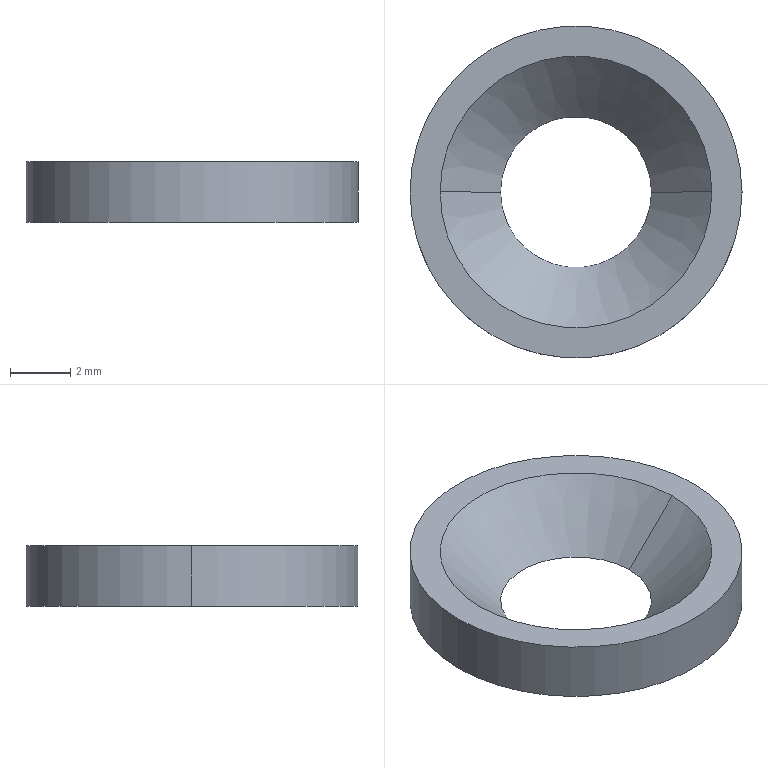Part | NX | features BREP 1 | 1 solid | 6 faces | box 11 x 11 x 2 mm | volume 111.003 mm3 | cone 2 | plane 2 | cylinder 2 | commonest cylinder face diameters 11 x2
STEP:
#1=CARTESIAN_POINT('',(-4.5,0.,2.));
#2=VERTEX_POINT('',#1);
#3=CARTESIAN_POINT('',(-2.5,0.,0.));
#4=VERTEX_POINT('',#3);
#5=CARTESIAN_POINT('',(-4.5,0.,2.));
#6=DIRECTION('',(-0.7071,0.,0.7071));
#7=VECTOR('',#6,1000.);
#8=LINE('',#5,#7);
#9=EDGE_CURVE('',#2,#4,#8,.F.);
#10=ORIENTED_EDGE('',*,*,#9,.T.);
#11=CARTESIAN_POINT('',(2.5,0.,0.));
#12=VERTEX_POINT('',#11);
#13=CARTESIAN_POINT('',(0.,0.,0.));
#14=DIRECTION('',(0.,0.,1.));
#15=DIRECTION('',(1.,0.,0.));
#16=AXIS2_PLACEMENT_3D('',#13,#14,#15);
#17=CIRCLE('',#16,2.5);
#18=EDGE_CURVE('',#12,#4,#17,.T.);
#19=ORIENTED_EDGE('',*,*,#18,.F.);
#20=CARTESIAN_POINT('',(4.5,0.,2.));
#21=VERTEX_POINT('',#20);
#22=CARTESIAN_POINT('',(4.5,0.,2.));
#23=DIRECTION('',(0.7071,0.,0.7071));
#24=VECTOR('',#23,1000.);
#25=LINE('',#22,#24);
#26=EDGE_CURVE('',#21,#12,#25,.F.);
#27=ORIENTED_EDGE('',*,*,#26,.F.);
#28=CARTESIAN_POINT('',(0.,0.,2.));
#29=DIRECTION('',(0.,0.,1.));
#30=DIRECTION('',(1.,0.,0.));
#31=AXIS2_PLACEMENT_3D('',#28,#29,#30);
#32=CIRCLE('',#31,4.5);
#33=EDGE_CURVE('',#21,#2,#32,.T.);
#34=ORIENTED_EDGE('',*,*,#33,.T.);
#35=EDGE_LOOP('',(#10,#19,#27,#34));
#36=FACE_BOUND('',#35,.T.);
#37=CARTESIAN_POINT('',(0.,0.,2.));
#38=DIRECTION('',(0.,0.,1.));
#39=DIRECTION('',(1.,0.,0.));
#40=AXIS2_PLACEMENT_3D('',#37,#38,#39);
#41=CONICAL_SURFACE('',#40,4.5,0.7854);
#42=ADVANCED_FACE('',(#36),#41,.F.);
#43=CARTESIAN_POINT('',(-5.5,0.,2.));
#44=VERTEX_POINT('',#43);
#45=CARTESIAN_POINT('',(5.5,0.,2.));
#46=VERTEX_POINT('',#45);
#47=CARTESIAN_POINT('',(0.,0.,2.));
#48=DIRECTION('',(0.,0.,1.));
#49=DIRECTION('',(1.,0.,0.));
#50=AXIS2_PLACEMENT_3D('',#47,#48,#49);
#51=CIRCLE('',#50,5.5);
#52=EDGE_CURVE('',#44,#46,#51,.T.);
#53=ORIENTED_EDGE('',*,*,#52,.T.);
#54=CARTESIAN_POINT('',(0.,0.,2.));
#55=DIRECTION('',(0.,0.,1.));
#56=DIRECTION('',(1.,0.,0.));
#57=AXIS2_PLACEMENT_3D('',#54,#55,#56);
#58=CIRCLE('',#57,5.5);
#59=EDGE_CURVE('',#46,#44,#58,.T.);
#60=ORIENTED_EDGE('',*,*,#59,.T.);
#61=EDGE_LOOP('',(#53,#60));
#62=FACE_BOUND('',#61,.T.);
#63=ORIENTED_EDGE('',*,*,#33,.F.);
#64=CARTESIAN_POINT('',(0.,0.,2.));
#65=DIRECTION('',(0.,0.,1.));
#66=DIRECTION('',(1.,0.,0.));
#67=AXIS2_PLACEMENT_3D('',#64,#65,#66);
#68=CIRCLE('',#67,4.5);
#69=EDGE_CURVE('',#2,#21,#68,.T.);
#70=ORIENTED_EDGE('',*,*,#69,.F.);
#71=EDGE_LOOP('',(#63,#70));
#72=FACE_BOUND('',#71,.T.);
#73=CARTESIAN_POINT('',(0.,0.,2.));
#74=DIRECTION('',(0.,0.,1.));
#75=DIRECTION('',(1.,0.,0.));
#76=AXIS2_PLACEMENT_3D('',#73,#74,#75);
#77=PLANE('',#76);
#78=ADVANCED_FACE('',(#62,#72),#77,.T.);
#79=CARTESIAN_POINT('',(5.5,0.,0.));
#80=VERTEX_POINT('',#79);
#81=CARTESIAN_POINT('',(5.5,0.,2.));
#82=DIRECTION('',(0.,0.,-1.));
#83=VECTOR('',#82,1000.);
#84=LINE('',#81,#83);
#85=EDGE_CURVE('',#46,#80,#84,.T.);
#86=ORIENTED_EDGE('',*,*,#85,.F.);
#87=ORIENTED_EDGE('',*,*,#52,.F.);
#88=CARTESIAN_POINT('',(-5.5,0.,0.));
#89=VERTEX_POINT('',#88);
#90=CARTESIAN_POINT('',(-5.5,0.,2.));
#91=DIRECTION('',(0.,0.,-1.));
#92=VECTOR('',#91,1000.);
#93=LINE('',#90,#92);
#94=EDGE_CURVE('',#44,#89,#93,.T.);
#95=ORIENTED_EDGE('',*,*,#94,.T.);
#96=CARTESIAN_POINT('',(0.,0.,0.));
#97=DIRECTION('',(0.,0.,1.));
#98=DIRECTION('',(1.,0.,0.));
#99=AXIS2_PLACEMENT_3D('',#96,#97,#98);
#100=CIRCLE('',#99,5.5);
#101=EDGE_CURVE('',#89,#80,#100,.T.);
#102=ORIENTED_EDGE('',*,*,#101,.T.);
#103=EDGE_LOOP('',(#86,#87,#95,#102));
#104=FACE_BOUND('',#103,.T.);
#105=CARTESIAN_POINT('',(0.,0.,2.));
#106=DIRECTION('',(0.,0.,-1.));
#107=DIRECTION('',(-1.,0.,0.));
#108=AXIS2_PLACEMENT_3D('',#105,#106,#107);
#109=CYLINDRICAL_SURFACE('',#108,5.5);
#110=ADVANCED_FACE('',(#104),#109,.T.);
#111=ORIENTED_EDGE('',*,*,#101,.F.);
#112=CARTESIAN_POINT('',(0.,0.,0.));
#113=DIRECTION('',(0.,0.,1.));
#114=DIRECTION('',(1.,0.,0.));
#115=AXIS2_PLACEMENT_3D('',#112,#113,#114);
#116=CIRCLE('',#115,5.5);
#117=EDGE_CURVE('',#80,#89,#116,.T.);
#118=ORIENTED_EDGE('',*,*,#117,.F.);
#119=EDGE_LOOP('',(#111,#118));
#120=FACE_BOUND('',#119,.T.);
#121=ORIENTED_EDGE('',*,*,#18,.T.);
#122=CARTESIAN_POINT('',(0.,0.,0.));
#123=DIRECTION('',(0.,0.,1.));
#124=DIRECTION('',(1.,0.,0.));
#125=AXIS2_PLACEMENT_3D('',#122,#123,#124);
#126=CIRCLE('',#125,2.5);
#127=EDGE_CURVE('',#4,#12,#126,.T.);
#128=ORIENTED_EDGE('',*,*,#127,.T.);
#129=EDGE_LOOP('',(#121,#128));
#130=FACE_BOUND('',#129,.T.);
#131=CARTESIAN_POINT('',(0.,0.,0.));
#132=DIRECTION('',(0.,0.,1.));
#133=DIRECTION('',(1.,0.,0.));
#134=AXIS2_PLACEMENT_3D('',#131,#132,#133);
#135=PLANE('',#134);
#136=ADVANCED_FACE('',(#120,#130),#135,.F.);
#137=ORIENTED_EDGE('',*,*,#59,.F.);
#138=ORIENTED_EDGE('',*,*,#85,.T.);
#139=ORIENTED_EDGE('',*,*,#117,.T.);
#140=ORIENTED_EDGE('',*,*,#94,.F.);
#141=EDGE_LOOP('',(#137,#138,#139,#140));
#142=FACE_BOUND('',#141,.T.);
#143=CARTESIAN_POINT('',(0.,0.,2.));
#144=DIRECTION('',(0.,0.,-1.));
#145=DIRECTION('',(-1.,0.,0.));
#146=AXIS2_PLACEMENT_3D('',#143,#144,#145);
#147=CYLINDRICAL_SURFACE('',#146,5.5);
#148=ADVANCED_FACE('',(#142),#147,.T.);
#149=ORIENTED_EDGE('',*,*,#127,.F.);
#150=ORIENTED_EDGE('',*,*,#9,.F.);
#151=ORIENTED_EDGE('',*,*,#69,.T.);
#152=ORIENTED_EDGE('',*,*,#26,.T.);
#153=EDGE_LOOP('',(#149,#150,#151,#152));
#154=FACE_BOUND('',#153,.T.);
#155=CARTESIAN_POINT('',(0.,0.,2.));
#156=DIRECTION('',(0.,0.,1.));
#157=DIRECTION('',(1.,0.,0.));
#158=AXIS2_PLACEMENT_3D('',#155,#156,#157);
#159=CONICAL_SURFACE('',#158,4.5,0.7854);
#160=ADVANCED_FACE('',(#154),#159,.F.);
#161=CLOSED_SHELL('',(#42,#78,#110,#136,#148,#160));
#162=MANIFOLD_SOLID_BREP('',#161);
#163=(LENGTH_UNIT()NAMED_UNIT(*)SI_UNIT(.MILLI.,.METRE.));
#164=UNCERTAINTY_MEASURE_WITH_UNIT(LENGTH_MEASURE(0.00001),#163,'','');
#165=(NAMED_UNIT(*)PLANE_ANGLE_UNIT()SI_UNIT($,.RADIAN.));
#166=(NAMED_UNIT(*)SI_UNIT($,.STERADIAN.)SOLID_ANGLE_UNIT());
#167=(GEOMETRIC_REPRESENTATION_CONTEXT(3)GLOBAL_UNCERTAINTY_ASSIGNED_CONTEXT((#164))GLOBAL_UNIT_ASSIGNED_CONTEXT((#163,#165,#166))REPRESENTATION_CONTEXT('',''));
#168=ADVANCED_BREP_SHAPE_REPRESENTATION('',(#162),#167);